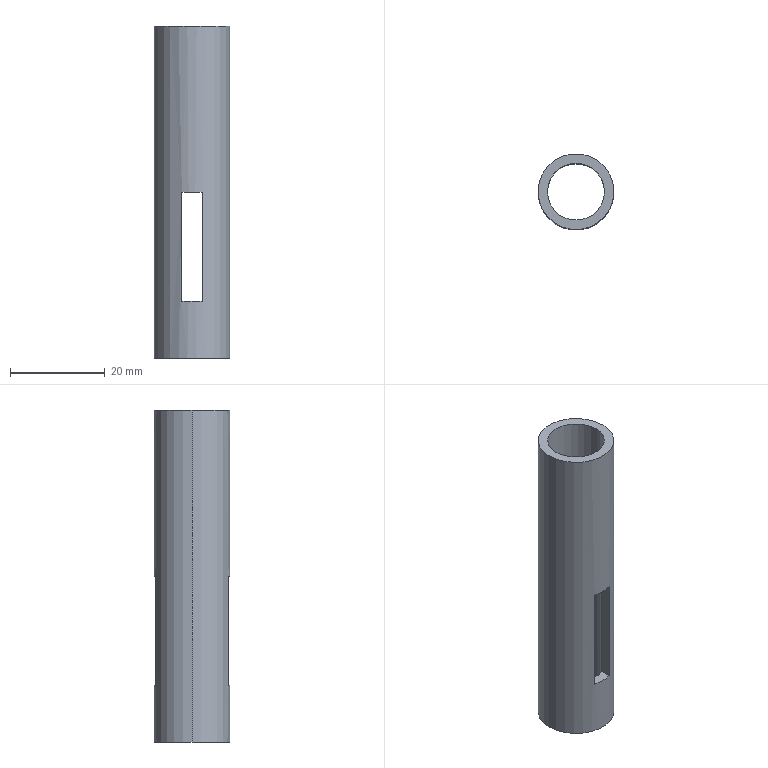Part | STEP file | Polisher lead screw | 1 solid | 14 faces | box 16 x 16 x 70 mm | volume 5755 mm3 | plane 10 | cylinder 4 | commonest cylinder face diameters 12 x2 16 x2
STEP:
#1=CARTESIAN_POINT('',(0.,0.,0.));
#2=DIRECTION('',(0.,0.,1.));
#3=DIRECTION('',(1.,0.,0.));
#4=AXIS2_PLACEMENT_3D('',#1,#2,#3);
#5=CARTESIAN_POINT('',(2.15,-5.602,-23.));
#6=VERTEX_POINT('',#5);
#7=CARTESIAN_POINT('',(-2.15,-5.602,-23.));
#8=VERTEX_POINT('',#7);
#9=CARTESIAN_POINT('',(0.,0.,-23.));
#10=DIRECTION('',(0.,0.,-1.));
#11=DIRECTION('',(-1.,0.,0.));
#12=AXIS2_PLACEMENT_3D('',#9,#10,#11);
#13=CIRCLE('',#12,6.);
#14=CARTESIAN_POINT('',(0.,0.,35.));
#15=DIRECTION('',(0.,0.,-1.));
#16=DIRECTION('',(-1.,0.,0.));
#17=AXIS2_PLACEMENT_3D('',#14,#15,#16);
#18=CYLINDRICAL_SURFACE('',#17,6.);
#19=CARTESIAN_POINT('',(0.,58.));
#20=DIRECTION('',(1.,0.));
#21=VECTOR('',#20,1.);
#22=LINE('',#19,#21);
#23=(GEOMETRIC_REPRESENTATION_CONTEXT(2)PARAMETRIC_REPRESENTATION_CONTEXT()REPRESENTATION_CONTEXT('',''));
#24=DEFINITIONAL_REPRESENTATION('',(#22),#23);
#25=PCURVE('',#18,#24);
#26=CARTESIAN_POINT('',(-2.15,-32.5,-23.));
#27=DIRECTION('',(0.,0.,-1.));
#28=DIRECTION('',(-1.,0.,0.));
#29=AXIS2_PLACEMENT_3D('',#26,#27,#28);
#30=PLANE('',#29);
#31=CARTESIAN_POINT('',(-2.15,32.5));
#32=DIRECTION('',(1.,0.));
#33=AXIS2_PLACEMENT_2D('',#31,#32);
#34=CIRCLE('',#33,6.);
#35=(GEOMETRIC_REPRESENTATION_CONTEXT(2)PARAMETRIC_REPRESENTATION_CONTEXT()REPRESENTATION_CONTEXT('',''));
#36=DEFINITIONAL_REPRESENTATION('',(#34),#35);
#37=PCURVE('',#30,#36);
#38=SURFACE_CURVE('',#13,(#25,#37),.PCURVE_S1.);
#39=EDGE_CURVE('',#6,#8,#38,.T.);
#40=ORIENTED_EDGE('',*,*,#39,.T.);
#41=CARTESIAN_POINT('',(-2.15,-5.602,0.));
#42=VERTEX_POINT('',#41);
#43=CARTESIAN_POINT('',(-2.15,-5.602,35.));
#44=DIRECTION('',(0.,0.,1.));
#45=VECTOR('',#44,1.);
#46=LINE('',#43,#45);
#47=CARTESIAN_POINT('',(5.079,0.));
#48=DIRECTION('',(0.,-1.));
#49=VECTOR('',#48,1.);
#50=LINE('',#47,#49);
#51=(GEOMETRIC_REPRESENTATION_CONTEXT(2)PARAMETRIC_REPRESENTATION_CONTEXT()REPRESENTATION_CONTEXT('',''));
#52=DEFINITIONAL_REPRESENTATION('',(#50),#51);
#53=PCURVE('',#18,#52);
#54=CARTESIAN_POINT('',(-2.15,-32.5,0.));
#55=DIRECTION('',(-1.,0.,0.));
#56=DIRECTION('',(0.,0.,1.));
#57=AXIS2_PLACEMENT_3D('',#54,#55,#56);
#58=PLANE('',#57);
#59=CARTESIAN_POINT('',(35.,26.898));
#60=DIRECTION('',(1.,0.));
#61=VECTOR('',#60,1.);
#62=LINE('',#59,#61);
#63=(GEOMETRIC_REPRESENTATION_CONTEXT(2)PARAMETRIC_REPRESENTATION_CONTEXT()REPRESENTATION_CONTEXT('',''));
#64=DEFINITIONAL_REPRESENTATION('',(#62),#63);
#65=PCURVE('',#58,#64);
#66=SURFACE_CURVE('',#46,(#53,#65),.PCURVE_S1.);
#67=EDGE_CURVE('',#8,#42,#66,.T.);
#68=ORIENTED_EDGE('',*,*,#67,.T.);
#69=CARTESIAN_POINT('',(2.15,-5.602,0.));
#70=VERTEX_POINT('',#69);
#71=CARTESIAN_POINT('',(0.,0.,0.));
#72=DIRECTION('',(0.,0.,1.));
#73=DIRECTION('',(1.,0.,0.));
#74=AXIS2_PLACEMENT_3D('',#71,#72,#73);
#75=CIRCLE('',#74,6.);
#76=CARTESIAN_POINT('',(9.425,35.));
#77=DIRECTION('',(-1.,0.));
#78=VECTOR('',#77,1.);
#79=LINE('',#76,#78);
#80=(GEOMETRIC_REPRESENTATION_CONTEXT(2)PARAMETRIC_REPRESENTATION_CONTEXT()REPRESENTATION_CONTEXT('',''));
#81=DEFINITIONAL_REPRESENTATION('',(#79),#80);
#82=PCURVE('',#18,#81);
#83=CARTESIAN_POINT('',(-2.15,-32.5,0.));
#84=DIRECTION('',(0.,0.,1.));
#85=DIRECTION('',(1.,0.,0.));
#86=AXIS2_PLACEMENT_3D('',#83,#84,#85);
#87=PLANE('',#86);
#88=CARTESIAN_POINT('',(2.15,32.5));
#89=DIRECTION('',(1.,0.));
#90=AXIS2_PLACEMENT_2D('',#88,#89);
#91=CIRCLE('',#90,6.);
#92=(GEOMETRIC_REPRESENTATION_CONTEXT(2)PARAMETRIC_REPRESENTATION_CONTEXT()REPRESENTATION_CONTEXT('',''));
#93=DEFINITIONAL_REPRESENTATION('',(#91),#92);
#94=PCURVE('',#87,#93);
#95=SURFACE_CURVE('',#75,(#82,#94),.PCURVE_S1.);
#96=EDGE_CURVE('',#42,#70,#95,.T.);
#97=ORIENTED_EDGE('',*,*,#96,.T.);
#98=CARTESIAN_POINT('',(2.15,-5.602,35.));
#99=DIRECTION('',(0.,0.,-1.));
#100=VECTOR('',#99,1.);
#101=LINE('',#98,#100);
#102=CARTESIAN_POINT('',(4.346,0.));
#103=DIRECTION('',(0.,1.));
#104=VECTOR('',#103,1.);
#105=LINE('',#102,#104);
#106=(GEOMETRIC_REPRESENTATION_CONTEXT(2)PARAMETRIC_REPRESENTATION_CONTEXT()REPRESENTATION_CONTEXT('',''));
#107=DEFINITIONAL_REPRESENTATION('',(#105),#106);
#108=PCURVE('',#18,#107);
#109=CARTESIAN_POINT('',(2.15,-32.5,0.));
#110=DIRECTION('',(1.,0.,0.));
#111=DIRECTION('',(0.,0.,-1.));
#112=AXIS2_PLACEMENT_3D('',#109,#110,#111);
#113=PLANE('',#112);
#114=CARTESIAN_POINT('',(-35.,26.898));
#115=DIRECTION('',(1.,0.));
#116=VECTOR('',#115,1.);
#117=LINE('',#114,#116);
#118=(GEOMETRIC_REPRESENTATION_CONTEXT(2)PARAMETRIC_REPRESENTATION_CONTEXT()REPRESENTATION_CONTEXT('',''));
#119=DEFINITIONAL_REPRESENTATION('',(#117),#118);
#120=PCURVE('',#113,#119);
#121=SURFACE_CURVE('',#101,(#108,#120),.PCURVE_S1.);
#122=EDGE_CURVE('',#70,#6,#121,.T.);
#123=ORIENTED_EDGE('',*,*,#122,.T.);
#124=EDGE_LOOP('',(#40,#68,#97,#123));
#125=FACE_BOUND('',#124,.F.);
#126=CARTESIAN_POINT('',(-6.,0.,35.));
#127=VERTEX_POINT('',#126);
#128=CARTESIAN_POINT('',(-6.,0.,-35.));
#129=VERTEX_POINT('',#128);
#130=CARTESIAN_POINT('',(-6.,0.,35.));
#131=DIRECTION('',(0.,0.,-1.));
#132=VECTOR('',#131,1.);
#133=LINE('',#130,#132);
#134=CARTESIAN_POINT('',(6.283,0.));
#135=DIRECTION('',(0.,1.));
#136=VECTOR('',#135,1.);
#137=LINE('',#134,#136);
#138=(GEOMETRIC_REPRESENTATION_CONTEXT(2)PARAMETRIC_REPRESENTATION_CONTEXT()REPRESENTATION_CONTEXT('',''));
#139=DEFINITIONAL_REPRESENTATION('',(#137),#138);
#140=PCURVE('',#18,#139);
#141=CARTESIAN_POINT('',(0.,0.,35.));
#142=DIRECTION('',(0.,0.,-1.));
#143=DIRECTION('',(-1.,0.,0.));
#144=AXIS2_PLACEMENT_3D('',#141,#142,#143);
#145=CYLINDRICAL_SURFACE('',#144,6.);
#146=CARTESIAN_POINT('',(0.,0.));
#147=DIRECTION('',(0.,1.));
#148=VECTOR('',#147,1.);
#149=LINE('',#146,#148);
#150=(GEOMETRIC_REPRESENTATION_CONTEXT(2)PARAMETRIC_REPRESENTATION_CONTEXT()REPRESENTATION_CONTEXT('',''));
#151=DEFINITIONAL_REPRESENTATION('',(#149),#150);
#152=PCURVE('',#145,#151);
#153=SURFACE_CURVE('',#133,(#140,#152),.PCURVE_S1.);
#154=EDGE_CURVE('',#127,#129,#153,.T.);
#155=ORIENTED_EDGE('',*,*,#154,.T.);
#156=CARTESIAN_POINT('',(6.,0.,-35.));
#157=VERTEX_POINT('',#156);
#158=CARTESIAN_POINT('',(0.,0.,-35.));
#159=DIRECTION('',(0.,0.,1.));
#160=DIRECTION('',(1.,0.,0.));
#161=AXIS2_PLACEMENT_3D('',#158,#159,#160);
#162=CIRCLE('',#161,6.);
#163=CARTESIAN_POINT('',(9.425,70.));
#164=DIRECTION('',(-1.,0.));
#165=VECTOR('',#164,1.);
#166=LINE('',#163,#165);
#167=(GEOMETRIC_REPRESENTATION_CONTEXT(2)PARAMETRIC_REPRESENTATION_CONTEXT()REPRESENTATION_CONTEXT('',''));
#168=DEFINITIONAL_REPRESENTATION('',(#166),#167);
#169=PCURVE('',#18,#168);
#170=CARTESIAN_POINT('',(0.,0.,-35.));
#171=DIRECTION('',(0.,0.,1.));
#172=DIRECTION('',(1.,0.,0.));
#173=AXIS2_PLACEMENT_3D('',#170,#171,#172);
#174=PLANE('',#173);
#175=CARTESIAN_POINT('',(0.,0.));
#176=DIRECTION('',(1.,0.));
#177=AXIS2_PLACEMENT_2D('',#175,#176);
#178=CIRCLE('',#177,6.);
#179=(GEOMETRIC_REPRESENTATION_CONTEXT(2)PARAMETRIC_REPRESENTATION_CONTEXT()REPRESENTATION_CONTEXT('',''));
#180=DEFINITIONAL_REPRESENTATION('',(#178),#179);
#181=PCURVE('',#174,#180);
#182=SURFACE_CURVE('',#162,(#169,#181),.PCURVE_S1.);
#183=EDGE_CURVE('',#129,#157,#182,.T.);
#184=ORIENTED_EDGE('',*,*,#183,.T.);
#185=CARTESIAN_POINT('',(6.,0.,35.));
#186=VERTEX_POINT('',#185);
#187=CARTESIAN_POINT('',(6.,0.,35.));
#188=DIRECTION('',(0.,0.,-1.));
#189=VECTOR('',#188,1.);
#190=LINE('',#187,#189);
#191=CARTESIAN_POINT('',(3.142,0.));
#192=DIRECTION('',(0.,1.));
#193=VECTOR('',#192,1.);
#194=LINE('',#191,#193);
#195=(GEOMETRIC_REPRESENTATION_CONTEXT(2)PARAMETRIC_REPRESENTATION_CONTEXT()REPRESENTATION_CONTEXT('',''));
#196=DEFINITIONAL_REPRESENTATION('',(#194),#195);
#197=PCURVE('',#18,#196);
#198=CARTESIAN_POINT('',(3.142,0.));
#199=DIRECTION('',(0.,1.));
#200=VECTOR('',#199,1.);
#201=LINE('',#198,#200);
#202=(GEOMETRIC_REPRESENTATION_CONTEXT(2)PARAMETRIC_REPRESENTATION_CONTEXT()REPRESENTATION_CONTEXT('',''));
#203=DEFINITIONAL_REPRESENTATION('',(#201),#202);
#204=PCURVE('',#145,#203);
#205=SURFACE_CURVE('',#190,(#197,#204),.PCURVE_S1.);
#206=EDGE_CURVE('',#186,#157,#205,.T.);
#207=ORIENTED_EDGE('',*,*,#206,.F.);
#208=CARTESIAN_POINT('',(0.,0.,35.));
#209=DIRECTION('',(0.,0.,1.));
#210=DIRECTION('',(1.,0.,0.));
#211=AXIS2_PLACEMENT_3D('',#208,#209,#210);
#212=CIRCLE('',#211,6.);
#213=CARTESIAN_POINT('',(9.425,0.));
#214=DIRECTION('',(-1.,0.));
#215=VECTOR('',#214,1.);
#216=LINE('',#213,#215);
#217=(GEOMETRIC_REPRESENTATION_CONTEXT(2)PARAMETRIC_REPRESENTATION_CONTEXT()REPRESENTATION_CONTEXT('',''));
#218=DEFINITIONAL_REPRESENTATION('',(#216),#217);
#219=PCURVE('',#18,#218);
#220=CARTESIAN_POINT('',(0.,0.,35.));
#221=DIRECTION('',(0.,0.,1.));
#222=DIRECTION('',(1.,0.,0.));
#223=AXIS2_PLACEMENT_3D('',#220,#221,#222);
#224=PLANE('',#223);
#225=CARTESIAN_POINT('',(0.,0.));
#226=DIRECTION('',(1.,0.));
#227=AXIS2_PLACEMENT_2D('',#225,#226);
#228=CIRCLE('',#227,6.);
#229=(GEOMETRIC_REPRESENTATION_CONTEXT(2)PARAMETRIC_REPRESENTATION_CONTEXT()REPRESENTATION_CONTEXT('',''));
#230=DEFINITIONAL_REPRESENTATION('',(#228),#229);
#231=PCURVE('',#224,#230);
#232=SURFACE_CURVE('',#212,(#219,#231),.PCURVE_S1.);
#233=EDGE_CURVE('',#127,#186,#232,.T.);
#234=ORIENTED_EDGE('',*,*,#233,.F.);
#235=EDGE_LOOP('',(#155,#184,#207,#234));
#236=FACE_BOUND('',#235,.F.);
#237=ADVANCED_FACE('',(#125,#236),#18,.F.);
#238=CARTESIAN_POINT('',(-2.15,7.706,-23.));
#239=VERTEX_POINT('',#238);
#240=CARTESIAN_POINT('',(2.15,7.706,-23.));
#241=VERTEX_POINT('',#240);
#242=CARTESIAN_POINT('',(0.,0.,-23.));
#243=DIRECTION('',(0.,0.,-1.));
#244=DIRECTION('',(-1.,0.,0.));
#245=AXIS2_PLACEMENT_3D('',#242,#243,#244);
#246=CIRCLE('',#245,8.);
#247=CARTESIAN_POINT('',(0.,0.,35.));
#248=DIRECTION('',(0.,0.,-1.));
#249=DIRECTION('',(-1.,0.,0.));
#250=AXIS2_PLACEMENT_3D('',#247,#248,#249);
#251=CYLINDRICAL_SURFACE('',#250,8.);
#252=CARTESIAN_POINT('',(0.,58.));
#253=DIRECTION('',(1.,0.));
#254=VECTOR('',#253,1.);
#255=LINE('',#252,#254);
#256=(GEOMETRIC_REPRESENTATION_CONTEXT(2)PARAMETRIC_REPRESENTATION_CONTEXT()REPRESENTATION_CONTEXT('',''));
#257=DEFINITIONAL_REPRESENTATION('',(#255),#256);
#258=PCURVE('',#251,#257);
#259=CARTESIAN_POINT('',(-2.15,-32.5,-23.));
#260=DIRECTION('',(0.,0.,-1.));
#261=DIRECTION('',(-1.,0.,0.));
#262=AXIS2_PLACEMENT_3D('',#259,#260,#261);
#263=PLANE('',#262);
#264=CARTESIAN_POINT('',(-2.15,32.5));
#265=DIRECTION('',(1.,0.));
#266=AXIS2_PLACEMENT_2D('',#264,#265);
#267=CIRCLE('',#266,8.);
#268=(GEOMETRIC_REPRESENTATION_CONTEXT(2)PARAMETRIC_REPRESENTATION_CONTEXT()REPRESENTATION_CONTEXT('',''));
#269=DEFINITIONAL_REPRESENTATION('',(#267),#268);
#270=PCURVE('',#263,#269);
#271=SURFACE_CURVE('',#246,(#258,#270),.PCURVE_S1.);
#272=EDGE_CURVE('',#239,#241,#271,.T.);
#273=ORIENTED_EDGE('',*,*,#272,.T.);
#274=CARTESIAN_POINT('',(2.15,7.706,0.));
#275=VERTEX_POINT('',#274);
#276=CARTESIAN_POINT('',(2.15,7.706,35.));
#277=DIRECTION('',(0.,0.,1.));
#278=VECTOR('',#277,1.);
#279=LINE('',#276,#278);
#280=CARTESIAN_POINT('',(1.843,0.));
#281=DIRECTION('',(0.,-1.));
#282=VECTOR('',#281,1.);
#283=LINE('',#280,#282);
#284=(GEOMETRIC_REPRESENTATION_CONTEXT(2)PARAMETRIC_REPRESENTATION_CONTEXT()REPRESENTATION_CONTEXT('',''));
#285=DEFINITIONAL_REPRESENTATION('',(#283),#284);
#286=PCURVE('',#251,#285);
#287=CARTESIAN_POINT('',(2.15,-32.5,0.));
#288=DIRECTION('',(1.,0.,0.));
#289=DIRECTION('',(0.,0.,-1.));
#290=AXIS2_PLACEMENT_3D('',#287,#288,#289);
#291=PLANE('',#290);
#292=CARTESIAN_POINT('',(-35.,40.206));
#293=DIRECTION('',(-1.,0.));
#294=VECTOR('',#293,1.);
#295=LINE('',#292,#294);
#296=(GEOMETRIC_REPRESENTATION_CONTEXT(2)PARAMETRIC_REPRESENTATION_CONTEXT()REPRESENTATION_CONTEXT('',''));
#297=DEFINITIONAL_REPRESENTATION('',(#295),#296);
#298=PCURVE('',#291,#297);
#299=SURFACE_CURVE('',#279,(#286,#298),.PCURVE_S1.);
#300=EDGE_CURVE('',#241,#275,#299,.T.);
#301=ORIENTED_EDGE('',*,*,#300,.T.);
#302=CARTESIAN_POINT('',(-2.15,7.706,0.));
#303=VERTEX_POINT('',#302);
#304=CARTESIAN_POINT('',(0.,0.,0.));
#305=DIRECTION('',(0.,0.,1.));
#306=DIRECTION('',(1.,0.,0.));
#307=AXIS2_PLACEMENT_3D('',#304,#305,#306);
#308=CIRCLE('',#307,8.);
#309=CARTESIAN_POINT('',(3.142,35.));
#310=DIRECTION('',(-1.,0.));
#311=VECTOR('',#310,1.);
#312=LINE('',#309,#311);
#313=(GEOMETRIC_REPRESENTATION_CONTEXT(2)PARAMETRIC_REPRESENTATION_CONTEXT()REPRESENTATION_CONTEXT('',''));
#314=DEFINITIONAL_REPRESENTATION('',(#312),#313);
#315=PCURVE('',#251,#314);
#316=CARTESIAN_POINT('',(-2.15,-32.5,0.));
#317=DIRECTION('',(0.,0.,1.));
#318=DIRECTION('',(1.,0.,0.));
#319=AXIS2_PLACEMENT_3D('',#316,#317,#318);
#320=PLANE('',#319);
#321=CARTESIAN_POINT('',(2.15,32.5));
#322=DIRECTION('',(1.,0.));
#323=AXIS2_PLACEMENT_2D('',#321,#322);
#324=CIRCLE('',#323,8.);
#325=(GEOMETRIC_REPRESENTATION_CONTEXT(2)PARAMETRIC_REPRESENTATION_CONTEXT()REPRESENTATION_CONTEXT('',''));
#326=DEFINITIONAL_REPRESENTATION('',(#324),#325);
#327=PCURVE('',#320,#326);
#328=SURFACE_CURVE('',#308,(#315,#327),.PCURVE_S1.);
#329=EDGE_CURVE('',#275,#303,#328,.T.);
#330=ORIENTED_EDGE('',*,*,#329,.T.);
#331=CARTESIAN_POINT('',(-2.15,7.706,35.));
#332=DIRECTION('',(0.,0.,-1.));
#333=VECTOR('',#332,1.);
#334=LINE('',#331,#333);
#335=CARTESIAN_POINT('',(1.299,0.));
#336=DIRECTION('',(0.,1.));
#337=VECTOR('',#336,1.);
#338=LINE('',#335,#337);
#339=(GEOMETRIC_REPRESENTATION_CONTEXT(2)PARAMETRIC_REPRESENTATION_CONTEXT()REPRESENTATION_CONTEXT('',''));
#340=DEFINITIONAL_REPRESENTATION('',(#338),#339);
#341=PCURVE('',#251,#340);
#342=CARTESIAN_POINT('',(-2.15,-32.5,0.));
#343=DIRECTION('',(-1.,0.,0.));
#344=DIRECTION('',(0.,0.,1.));
#345=AXIS2_PLACEMENT_3D('',#342,#343,#344);
#346=PLANE('',#345);
#347=CARTESIAN_POINT('',(35.,40.206));
#348=DIRECTION('',(-1.,0.));
#349=VECTOR('',#348,1.);
#350=LINE('',#347,#349);
#351=(GEOMETRIC_REPRESENTATION_CONTEXT(2)PARAMETRIC_REPRESENTATION_CONTEXT()REPRESENTATION_CONTEXT('',''));
#352=DEFINITIONAL_REPRESENTATION('',(#350),#351);
#353=PCURVE('',#346,#352);
#354=SURFACE_CURVE('',#334,(#341,#353),.PCURVE_S1.);
#355=EDGE_CURVE('',#303,#239,#354,.T.);
#356=ORIENTED_EDGE('',*,*,#355,.T.);
#357=EDGE_LOOP('',(#273,#301,#330,#356));
#358=FACE_BOUND('',#357,.T.);
#359=CARTESIAN_POINT('',(8.,0.,35.));
#360=VERTEX_POINT('',#359);
#361=CARTESIAN_POINT('',(-8.,0.,35.));
#362=VERTEX_POINT('',#361);
#363=CARTESIAN_POINT('',(0.,0.,35.));
#364=DIRECTION('',(0.,0.,1.));
#365=DIRECTION('',(1.,0.,0.));
#366=AXIS2_PLACEMENT_3D('',#363,#364,#365);
#367=CIRCLE('',#366,8.);
#368=CARTESIAN_POINT('',(3.142,0.));
#369=DIRECTION('',(-1.,0.));
#370=VECTOR('',#369,1.);
#371=LINE('',#368,#370);
#372=(GEOMETRIC_REPRESENTATION_CONTEXT(2)PARAMETRIC_REPRESENTATION_CONTEXT()REPRESENTATION_CONTEXT('',''));
#373=DEFINITIONAL_REPRESENTATION('',(#371),#372);
#374=PCURVE('',#251,#373);
#375=CARTESIAN_POINT('',(0.,0.));
#376=DIRECTION('',(1.,0.));
#377=AXIS2_PLACEMENT_2D('',#375,#376);
#378=CIRCLE('',#377,8.);
#379=(GEOMETRIC_REPRESENTATION_CONTEXT(2)PARAMETRIC_REPRESENTATION_CONTEXT()REPRESENTATION_CONTEXT('',''));
#380=DEFINITIONAL_REPRESENTATION('',(#378),#379);
#381=PCURVE('',#224,#380);
#382=SURFACE_CURVE('',#367,(#374,#381),.PCURVE_S1.);
#383=EDGE_CURVE('',#360,#362,#382,.T.);
#384=ORIENTED_EDGE('',*,*,#383,.F.);
#385=CARTESIAN_POINT('',(8.,0.,-35.));
#386=VERTEX_POINT('',#385);
#387=CARTESIAN_POINT('',(8.,0.,35.));
#388=DIRECTION('',(0.,0.,-1.));
#389=VECTOR('',#388,1.);
#390=LINE('',#387,#389);
#391=CARTESIAN_POINT('',(3.142,0.));
#392=DIRECTION('',(0.,1.));
#393=VECTOR('',#392,1.);
#394=LINE('',#391,#393);
#395=(GEOMETRIC_REPRESENTATION_CONTEXT(2)PARAMETRIC_REPRESENTATION_CONTEXT()REPRESENTATION_CONTEXT('',''));
#396=DEFINITIONAL_REPRESENTATION('',(#394),#395);
#397=PCURVE('',#251,#396);
#398=CARTESIAN_POINT('',(0.,0.,35.));
#399=DIRECTION('',(0.,0.,-1.));
#400=DIRECTION('',(-1.,0.,0.));
#401=AXIS2_PLACEMENT_3D('',#398,#399,#400);
#402=CYLINDRICAL_SURFACE('',#401,8.);
#403=CARTESIAN_POINT('',(3.142,0.));
#404=DIRECTION('',(0.,1.));
#405=VECTOR('',#404,1.);
#406=LINE('',#403,#405);
#407=(GEOMETRIC_REPRESENTATION_CONTEXT(2)PARAMETRIC_REPRESENTATION_CONTEXT()REPRESENTATION_CONTEXT('',''));
#408=DEFINITIONAL_REPRESENTATION('',(#406),#407);
#409=PCURVE('',#402,#408);
#410=SURFACE_CURVE('',#390,(#397,#409),.PCURVE_S1.);
#411=EDGE_CURVE('',#360,#386,#410,.T.);
#412=ORIENTED_EDGE('',*,*,#411,.T.);
#413=CARTESIAN_POINT('',(-8.,0.,-35.));
#414=VERTEX_POINT('',#413);
#415=CARTESIAN_POINT('',(0.,0.,-35.));
#416=DIRECTION('',(0.,0.,1.));
#417=DIRECTION('',(1.,0.,0.));
#418=AXIS2_PLACEMENT_3D('',#415,#416,#417);
#419=CIRCLE('',#418,8.);
#420=CARTESIAN_POINT('',(3.142,70.));
#421=DIRECTION('',(-1.,0.));
#422=VECTOR('',#421,1.);
#423=LINE('',#420,#422);
#424=(GEOMETRIC_REPRESENTATION_CONTEXT(2)PARAMETRIC_REPRESENTATION_CONTEXT()REPRESENTATION_CONTEXT('',''));
#425=DEFINITIONAL_REPRESENTATION('',(#423),#424);
#426=PCURVE('',#251,#425);
#427=CARTESIAN_POINT('',(0.,0.));
#428=DIRECTION('',(1.,0.));
#429=AXIS2_PLACEMENT_2D('',#427,#428);
#430=CIRCLE('',#429,8.);
#431=(GEOMETRIC_REPRESENTATION_CONTEXT(2)PARAMETRIC_REPRESENTATION_CONTEXT()REPRESENTATION_CONTEXT('',''));
#432=DEFINITIONAL_REPRESENTATION('',(#430),#431);
#433=PCURVE('',#174,#432);
#434=SURFACE_CURVE('',#419,(#426,#433),.PCURVE_S1.);
#435=EDGE_CURVE('',#386,#414,#434,.T.);
#436=ORIENTED_EDGE('',*,*,#435,.T.);
#437=CARTESIAN_POINT('',(-8.,0.,35.));
#438=DIRECTION('',(0.,0.,-1.));
#439=VECTOR('',#438,1.);
#440=LINE('',#437,#439);
#441=CARTESIAN_POINT('',(0.,0.));
#442=DIRECTION('',(0.,1.));
#443=VECTOR('',#442,1.);
#444=LINE('',#441,#443);
#445=(GEOMETRIC_REPRESENTATION_CONTEXT(2)PARAMETRIC_REPRESENTATION_CONTEXT()REPRESENTATION_CONTEXT('',''));
#446=DEFINITIONAL_REPRESENTATION('',(#444),#445);
#447=PCURVE('',#251,#446);
#448=CARTESIAN_POINT('',(6.283,0.));
#449=DIRECTION('',(0.,1.));
#450=VECTOR('',#449,1.);
#451=LINE('',#448,#450);
#452=(GEOMETRIC_REPRESENTATION_CONTEXT(2)PARAMETRIC_REPRESENTATION_CONTEXT()REPRESENTATION_CONTEXT('',''));
#453=DEFINITIONAL_REPRESENTATION('',(#451),#452);
#454=PCURVE('',#402,#453);
#455=SURFACE_CURVE('',#440,(#447,#454),.PCURVE_S1.);
#456=EDGE_CURVE('',#362,#414,#455,.T.);
#457=ORIENTED_EDGE('',*,*,#456,.F.);
#458=EDGE_LOOP('',(#384,#412,#436,#457));
#459=FACE_BOUND('',#458,.T.);
#460=ADVANCED_FACE('',(#358,#459),#251,.T.);
#461=CARTESIAN_POINT('',(0.,0.,35.));
#462=DIRECTION('',(0.,0.,1.));
#463=DIRECTION('',(1.,0.,0.));
#464=AXIS2_PLACEMENT_3D('',#461,#462,#463);
#465=CIRCLE('',#464,8.);
#466=CARTESIAN_POINT('',(0.,0.));
#467=DIRECTION('',(1.,0.));
#468=AXIS2_PLACEMENT_2D('',#466,#467);
#469=CIRCLE('',#468,8.);
#470=(GEOMETRIC_REPRESENTATION_CONTEXT(2)PARAMETRIC_REPRESENTATION_CONTEXT()REPRESENTATION_CONTEXT('',''));
#471=DEFINITIONAL_REPRESENTATION('',(#469),#470);
#472=PCURVE('',#224,#471);
#473=CARTESIAN_POINT('',(9.425,0.));
#474=DIRECTION('',(-1.,0.));
#475=VECTOR('',#474,1.);
#476=LINE('',#473,#475);
#477=(GEOMETRIC_REPRESENTATION_CONTEXT(2)PARAMETRIC_REPRESENTATION_CONTEXT()REPRESENTATION_CONTEXT('',''));
#478=DEFINITIONAL_REPRESENTATION('',(#476),#477);
#479=PCURVE('',#402,#478);
#480=SURFACE_CURVE('',#465,(#472,#479),.PCURVE_S1.);
#481=EDGE_CURVE('',#362,#360,#480,.T.);
#482=ORIENTED_EDGE('',*,*,#481,.T.);
#483=ORIENTED_EDGE('',*,*,#383,.T.);
#484=EDGE_LOOP('',(#482,#483));
#485=FACE_BOUND('',#484,.T.);
#486=ORIENTED_EDGE('',*,*,#233,.F.);
#487=CARTESIAN_POINT('',(0.,0.,35.));
#488=DIRECTION('',(0.,0.,1.));
#489=DIRECTION('',(1.,0.,0.));
#490=AXIS2_PLACEMENT_3D('',#487,#488,#489);
#491=CIRCLE('',#490,6.);
#492=CARTESIAN_POINT('',(0.,0.));
#493=DIRECTION('',(1.,0.));
#494=AXIS2_PLACEMENT_2D('',#492,#493);
#495=CIRCLE('',#494,6.);
#496=(GEOMETRIC_REPRESENTATION_CONTEXT(2)PARAMETRIC_REPRESENTATION_CONTEXT()REPRESENTATION_CONTEXT('',''));
#497=DEFINITIONAL_REPRESENTATION('',(#495),#496);
#498=PCURVE('',#224,#497);
#499=CARTESIAN_POINT('',(3.142,0.));
#500=DIRECTION('',(-1.,0.));
#501=VECTOR('',#500,1.);
#502=LINE('',#499,#501);
#503=(GEOMETRIC_REPRESENTATION_CONTEXT(2)PARAMETRIC_REPRESENTATION_CONTEXT()REPRESENTATION_CONTEXT('',''));
#504=DEFINITIONAL_REPRESENTATION('',(#502),#503);
#505=PCURVE('',#145,#504);
#506=SURFACE_CURVE('',#491,(#498,#505),.PCURVE_S1.);
#507=EDGE_CURVE('',#186,#127,#506,.T.);
#508=ORIENTED_EDGE('',*,*,#507,.F.);
#509=EDGE_LOOP('',(#486,#508));
#510=FACE_BOUND('',#509,.T.);
#511=ADVANCED_FACE('',(#485,#510),#224,.T.);
#512=CARTESIAN_POINT('',(0.,0.,-35.));
#513=DIRECTION('',(0.,0.,1.));
#514=DIRECTION('',(1.,0.,0.));
#515=AXIS2_PLACEMENT_3D('',#512,#513,#514);
#516=CIRCLE('',#515,8.);
#517=CARTESIAN_POINT('',(0.,0.));
#518=DIRECTION('',(1.,0.));
#519=AXIS2_PLACEMENT_2D('',#517,#518);
#520=CIRCLE('',#519,8.);
#521=(GEOMETRIC_REPRESENTATION_CONTEXT(2)PARAMETRIC_REPRESENTATION_CONTEXT()REPRESENTATION_CONTEXT('',''));
#522=DEFINITIONAL_REPRESENTATION('',(#520),#521);
#523=PCURVE('',#174,#522);
#524=CARTESIAN_POINT('',(9.425,70.));
#525=DIRECTION('',(-1.,0.));
#526=VECTOR('',#525,1.);
#527=LINE('',#524,#526);
#528=(GEOMETRIC_REPRESENTATION_CONTEXT(2)PARAMETRIC_REPRESENTATION_CONTEXT()REPRESENTATION_CONTEXT('',''));
#529=DEFINITIONAL_REPRESENTATION('',(#527),#528);
#530=PCURVE('',#402,#529);
#531=SURFACE_CURVE('',#516,(#523,#530),.PCURVE_S1.);
#532=EDGE_CURVE('',#414,#386,#531,.T.);
#533=ORIENTED_EDGE('',*,*,#532,.F.);
#534=ORIENTED_EDGE('',*,*,#435,.F.);
#535=EDGE_LOOP('',(#533,#534));
#536=FACE_BOUND('',#535,.T.);
#537=ORIENTED_EDGE('',*,*,#183,.T.);
#538=CARTESIAN_POINT('',(0.,0.,-35.));
#539=DIRECTION('',(0.,0.,1.));
#540=DIRECTION('',(1.,0.,0.));
#541=AXIS2_PLACEMENT_3D('',#538,#539,#540);
#542=CIRCLE('',#541,6.);
#543=CARTESIAN_POINT('',(0.,0.));
#544=DIRECTION('',(1.,0.));
#545=AXIS2_PLACEMENT_2D('',#543,#544);
#546=CIRCLE('',#545,6.);
#547=(GEOMETRIC_REPRESENTATION_CONTEXT(2)PARAMETRIC_REPRESENTATION_CONTEXT()REPRESENTATION_CONTEXT('',''));
#548=DEFINITIONAL_REPRESENTATION('',(#546),#547);
#549=PCURVE('',#174,#548);
#550=CARTESIAN_POINT('',(3.142,70.));
#551=DIRECTION('',(-1.,0.));
#552=VECTOR('',#551,1.);
#553=LINE('',#550,#552);
#554=(GEOMETRIC_REPRESENTATION_CONTEXT(2)PARAMETRIC_REPRESENTATION_CONTEXT()REPRESENTATION_CONTEXT('',''));
#555=DEFINITIONAL_REPRESENTATION('',(#553),#554);
#556=PCURVE('',#145,#555);
#557=SURFACE_CURVE('',#542,(#549,#556),.PCURVE_S1.);
#558=EDGE_CURVE('',#157,#129,#557,.T.);
#559=ORIENTED_EDGE('',*,*,#558,.T.);
#560=EDGE_LOOP('',(#537,#559));
#561=FACE_BOUND('',#560,.T.);
#562=ADVANCED_FACE('',(#536,#561),#174,.F.);
#563=ORIENTED_EDGE('',*,*,#411,.F.);
#564=ORIENTED_EDGE('',*,*,#481,.F.);
#565=ORIENTED_EDGE('',*,*,#456,.T.);
#566=ORIENTED_EDGE('',*,*,#532,.T.);
#567=EDGE_LOOP('',(#563,#564,#565,#566));
#568=FACE_BOUND('',#567,.T.);
#569=CARTESIAN_POINT('',(-2.15,-7.706,0.));
#570=VERTEX_POINT('',#569);
#571=CARTESIAN_POINT('',(2.15,-7.706,0.));
#572=VERTEX_POINT('',#571);
#573=CARTESIAN_POINT('',(0.,0.,0.));
#574=DIRECTION('',(0.,0.,1.));
#575=DIRECTION('',(1.,0.,0.));
#576=AXIS2_PLACEMENT_3D('',#573,#574,#575);
#577=CIRCLE('',#576,8.);
#578=CARTESIAN_POINT('',(9.425,35.));
#579=DIRECTION('',(-1.,0.));
#580=VECTOR('',#579,1.);
#581=LINE('',#578,#580);
#582=(GEOMETRIC_REPRESENTATION_CONTEXT(2)PARAMETRIC_REPRESENTATION_CONTEXT()REPRESENTATION_CONTEXT('',''));
#583=DEFINITIONAL_REPRESENTATION('',(#581),#582);
#584=PCURVE('',#402,#583);
#585=CARTESIAN_POINT('',(2.15,32.5));
#586=DIRECTION('',(1.,0.));
#587=AXIS2_PLACEMENT_2D('',#585,#586);
#588=CIRCLE('',#587,8.);
#589=(GEOMETRIC_REPRESENTATION_CONTEXT(2)PARAMETRIC_REPRESENTATION_CONTEXT()REPRESENTATION_CONTEXT('',''));
#590=DEFINITIONAL_REPRESENTATION('',(#588),#589);
#591=PCURVE('',#87,#590);
#592=SURFACE_CURVE('',#577,(#584,#591),.PCURVE_S1.);
#593=EDGE_CURVE('',#570,#572,#592,.T.);
#594=ORIENTED_EDGE('',*,*,#593,.T.);
#595=CARTESIAN_POINT('',(2.15,-7.706,-23.));
#596=VERTEX_POINT('',#595);
#597=CARTESIAN_POINT('',(2.15,-7.706,35.));
#598=DIRECTION('',(0.,0.,-1.));
#599=VECTOR('',#598,1.);
#600=LINE('',#597,#599);
#601=CARTESIAN_POINT('',(4.44,0.));
#602=DIRECTION('',(0.,1.));
#603=VECTOR('',#602,1.);
#604=LINE('',#601,#603);
#605=(GEOMETRIC_REPRESENTATION_CONTEXT(2)PARAMETRIC_REPRESENTATION_CONTEXT()REPRESENTATION_CONTEXT('',''));
#606=DEFINITIONAL_REPRESENTATION('',(#604),#605);
#607=PCURVE('',#402,#606);
#608=CARTESIAN_POINT('',(-35.,24.794));
#609=DIRECTION('',(1.,0.));
#610=VECTOR('',#609,1.);
#611=LINE('',#608,#610);
#612=(GEOMETRIC_REPRESENTATION_CONTEXT(2)PARAMETRIC_REPRESENTATION_CONTEXT()REPRESENTATION_CONTEXT('',''));
#613=DEFINITIONAL_REPRESENTATION('',(#611),#612);
#614=PCURVE('',#113,#613);
#615=SURFACE_CURVE('',#600,(#607,#614),.PCURVE_S1.);
#616=EDGE_CURVE('',#572,#596,#615,.T.);
#617=ORIENTED_EDGE('',*,*,#616,.T.);
#618=CARTESIAN_POINT('',(-2.15,-7.706,-23.));
#619=VERTEX_POINT('',#618);
#620=CARTESIAN_POINT('',(0.,0.,-23.));
#621=DIRECTION('',(0.,0.,-1.));
#622=DIRECTION('',(-1.,0.,0.));
#623=AXIS2_PLACEMENT_3D('',#620,#621,#622);
#624=CIRCLE('',#623,8.);
#625=CARTESIAN_POINT('',(0.,58.));
#626=DIRECTION('',(1.,0.));
#627=VECTOR('',#626,1.);
#628=LINE('',#625,#627);
#629=(GEOMETRIC_REPRESENTATION_CONTEXT(2)PARAMETRIC_REPRESENTATION_CONTEXT()REPRESENTATION_CONTEXT('',''));
#630=DEFINITIONAL_REPRESENTATION('',(#628),#629);
#631=PCURVE('',#402,#630);
#632=CARTESIAN_POINT('',(-2.15,32.5));
#633=DIRECTION('',(1.,0.));
#634=AXIS2_PLACEMENT_2D('',#632,#633);
#635=CIRCLE('',#634,8.);
#636=(GEOMETRIC_REPRESENTATION_CONTEXT(2)PARAMETRIC_REPRESENTATION_CONTEXT()REPRESENTATION_CONTEXT('',''));
#637=DEFINITIONAL_REPRESENTATION('',(#635),#636);
#638=PCURVE('',#30,#637);
#639=SURFACE_CURVE('',#624,(#631,#638),.PCURVE_S1.);
#640=EDGE_CURVE('',#596,#619,#639,.T.);
#641=ORIENTED_EDGE('',*,*,#640,.T.);
#642=CARTESIAN_POINT('',(-2.15,-7.706,35.));
#643=DIRECTION('',(0.,0.,1.));
#644=VECTOR('',#643,1.);
#645=LINE('',#642,#644);
#646=CARTESIAN_POINT('',(4.984,0.));
#647=DIRECTION('',(0.,-1.));
#648=VECTOR('',#647,1.);
#649=LINE('',#646,#648);
#650=(GEOMETRIC_REPRESENTATION_CONTEXT(2)PARAMETRIC_REPRESENTATION_CONTEXT()REPRESENTATION_CONTEXT('',''));
#651=DEFINITIONAL_REPRESENTATION('',(#649),#650);
#652=PCURVE('',#402,#651);
#653=CARTESIAN_POINT('',(35.,24.794));
#654=DIRECTION('',(1.,0.));
#655=VECTOR('',#654,1.);
#656=LINE('',#653,#655);
#657=(GEOMETRIC_REPRESENTATION_CONTEXT(2)PARAMETRIC_REPRESENTATION_CONTEXT()REPRESENTATION_CONTEXT('',''));
#658=DEFINITIONAL_REPRESENTATION('',(#656),#657);
#659=PCURVE('',#58,#658);
#660=SURFACE_CURVE('',#645,(#652,#659),.PCURVE_S1.);
#661=EDGE_CURVE('',#619,#570,#660,.T.);
#662=ORIENTED_EDGE('',*,*,#661,.T.);
#663=EDGE_LOOP('',(#594,#617,#641,#662));
#664=FACE_BOUND('',#663,.T.);
#665=ADVANCED_FACE('',(#568,#664),#402,.T.);
#666=ORIENTED_EDGE('',*,*,#558,.T.);
#667=ORIENTED_EDGE('',*,*,#154,.F.);
#668=ORIENTED_EDGE('',*,*,#507,.F.);
#669=ORIENTED_EDGE('',*,*,#206,.T.);
#670=EDGE_LOOP('',(#666,#667,#668,#669));
#671=FACE_BOUND('',#670,.F.);
#672=CARTESIAN_POINT('',(2.15,5.602,0.));
#673=VERTEX_POINT('',#672);
#674=CARTESIAN_POINT('',(-2.15,5.602,0.));
#675=VERTEX_POINT('',#674);
#676=CARTESIAN_POINT('',(0.,0.,0.));
#677=DIRECTION('',(0.,0.,1.));
#678=DIRECTION('',(1.,0.,0.));
#679=AXIS2_PLACEMENT_3D('',#676,#677,#678);
#680=CIRCLE('',#679,6.);
#681=CARTESIAN_POINT('',(3.142,35.));
#682=DIRECTION('',(-1.,0.));
#683=VECTOR('',#682,1.);
#684=LINE('',#681,#683);
#685=(GEOMETRIC_REPRESENTATION_CONTEXT(2)PARAMETRIC_REPRESENTATION_CONTEXT()REPRESENTATION_CONTEXT('',''));
#686=DEFINITIONAL_REPRESENTATION('',(#684),#685);
#687=PCURVE('',#145,#686);
#688=CARTESIAN_POINT('',(2.15,32.5));
#689=DIRECTION('',(1.,0.));
#690=AXIS2_PLACEMENT_2D('',#688,#689);
#691=CIRCLE('',#690,6.);
#692=(GEOMETRIC_REPRESENTATION_CONTEXT(2)PARAMETRIC_REPRESENTATION_CONTEXT()REPRESENTATION_CONTEXT('',''));
#693=DEFINITIONAL_REPRESENTATION('',(#691),#692);
#694=PCURVE('',#320,#693);
#695=SURFACE_CURVE('',#680,(#687,#694),.PCURVE_S1.);
#696=EDGE_CURVE('',#673,#675,#695,.T.);
#697=ORIENTED_EDGE('',*,*,#696,.T.);
#698=CARTESIAN_POINT('',(-2.15,5.602,-23.));
#699=VERTEX_POINT('',#698);
#700=CARTESIAN_POINT('',(-2.15,5.602,35.));
#701=DIRECTION('',(0.,0.,-1.));
#702=VECTOR('',#701,1.);
#703=LINE('',#700,#702);
#704=CARTESIAN_POINT('',(1.204,0.));
#705=DIRECTION('',(0.,1.));
#706=VECTOR('',#705,1.);
#707=LINE('',#704,#706);
#708=(GEOMETRIC_REPRESENTATION_CONTEXT(2)PARAMETRIC_REPRESENTATION_CONTEXT()REPRESENTATION_CONTEXT('',''));
#709=DEFINITIONAL_REPRESENTATION('',(#707),#708);
#710=PCURVE('',#145,#709);
#711=CARTESIAN_POINT('',(35.,38.102));
#712=DIRECTION('',(-1.,0.));
#713=VECTOR('',#712,1.);
#714=LINE('',#711,#713);
#715=(GEOMETRIC_REPRESENTATION_CONTEXT(2)PARAMETRIC_REPRESENTATION_CONTEXT()REPRESENTATION_CONTEXT('',''));
#716=DEFINITIONAL_REPRESENTATION('',(#714),#715);
#717=PCURVE('',#346,#716);
#718=SURFACE_CURVE('',#703,(#710,#717),.PCURVE_S1.);
#719=EDGE_CURVE('',#675,#699,#718,.T.);
#720=ORIENTED_EDGE('',*,*,#719,.T.);
#721=CARTESIAN_POINT('',(2.15,5.602,-23.));
#722=VERTEX_POINT('',#721);
#723=CARTESIAN_POINT('',(0.,0.,-23.));
#724=DIRECTION('',(0.,0.,-1.));
#725=DIRECTION('',(-1.,0.,0.));
#726=AXIS2_PLACEMENT_3D('',#723,#724,#725);
#727=CIRCLE('',#726,6.);
#728=CARTESIAN_POINT('',(0.,58.));
#729=DIRECTION('',(1.,0.));
#730=VECTOR('',#729,1.);
#731=LINE('',#728,#730);
#732=(GEOMETRIC_REPRESENTATION_CONTEXT(2)PARAMETRIC_REPRESENTATION_CONTEXT()REPRESENTATION_CONTEXT('',''));
#733=DEFINITIONAL_REPRESENTATION('',(#731),#732);
#734=PCURVE('',#145,#733);
#735=CARTESIAN_POINT('',(-2.15,32.5));
#736=DIRECTION('',(1.,0.));
#737=AXIS2_PLACEMENT_2D('',#735,#736);
#738=CIRCLE('',#737,6.);
#739=(GEOMETRIC_REPRESENTATION_CONTEXT(2)PARAMETRIC_REPRESENTATION_CONTEXT()REPRESENTATION_CONTEXT('',''));
#740=DEFINITIONAL_REPRESENTATION('',(#738),#739);
#741=PCURVE('',#263,#740);
#742=SURFACE_CURVE('',#727,(#734,#741),.PCURVE_S1.);
#743=EDGE_CURVE('',#699,#722,#742,.T.);
#744=ORIENTED_EDGE('',*,*,#743,.T.);
#745=CARTESIAN_POINT('',(2.15,5.602,35.));
#746=DIRECTION('',(0.,0.,1.));
#747=VECTOR('',#746,1.);
#748=LINE('',#745,#747);
#749=CARTESIAN_POINT('',(1.937,0.));
#750=DIRECTION('',(0.,-1.));
#751=VECTOR('',#750,1.);
#752=LINE('',#749,#751);
#753=(GEOMETRIC_REPRESENTATION_CONTEXT(2)PARAMETRIC_REPRESENTATION_CONTEXT()REPRESENTATION_CONTEXT('',''));
#754=DEFINITIONAL_REPRESENTATION('',(#752),#753);
#755=PCURVE('',#145,#754);
#756=CARTESIAN_POINT('',(-35.,38.102));
#757=DIRECTION('',(-1.,0.));
#758=VECTOR('',#757,1.);
#759=LINE('',#756,#758);
#760=(GEOMETRIC_REPRESENTATION_CONTEXT(2)PARAMETRIC_REPRESENTATION_CONTEXT()REPRESENTATION_CONTEXT('',''));
#761=DEFINITIONAL_REPRESENTATION('',(#759),#760);
#762=PCURVE('',#291,#761);
#763=SURFACE_CURVE('',#748,(#755,#762),.PCURVE_S1.);
#764=EDGE_CURVE('',#722,#673,#763,.T.);
#765=ORIENTED_EDGE('',*,*,#764,.T.);
#766=EDGE_LOOP('',(#697,#720,#744,#765));
#767=FACE_BOUND('',#766,.F.);
#768=ADVANCED_FACE('',(#671,#767),#145,.F.);
#769=CARTESIAN_POINT('',(2.15,-32.5,-23.));
#770=DIRECTION('',(0.,1.,0.));
#771=VECTOR('',#770,1.);
#772=LINE('',#769,#771);
#773=CARTESIAN_POINT('',(-4.3,0.));
#774=DIRECTION('',(0.,1.));
#775=VECTOR('',#774,1.);
#776=LINE('',#773,#775);
#777=(GEOMETRIC_REPRESENTATION_CONTEXT(2)PARAMETRIC_REPRESENTATION_CONTEXT()REPRESENTATION_CONTEXT('',''));
#778=DEFINITIONAL_REPRESENTATION('',(#776),#777);
#779=PCURVE('',#30,#778);
#780=CARTESIAN_POINT('',(23.,0.));
#781=DIRECTION('',(0.,1.));
#782=VECTOR('',#781,1.);
#783=LINE('',#780,#782);
#784=(GEOMETRIC_REPRESENTATION_CONTEXT(2)PARAMETRIC_REPRESENTATION_CONTEXT()REPRESENTATION_CONTEXT('',''));
#785=DEFINITIONAL_REPRESENTATION('',(#783),#784);
#786=PCURVE('',#113,#785);
#787=SURFACE_CURVE('',#772,(#779,#786),.PCURVE_S1.);
#788=EDGE_CURVE('',#596,#6,#787,.T.);
#789=ORIENTED_EDGE('',*,*,#788,.T.);
#790=ORIENTED_EDGE('',*,*,#39,.T.);
#791=CARTESIAN_POINT('',(-2.15,-32.5,-23.));
#792=DIRECTION('',(0.,1.,0.));
#793=VECTOR('',#792,1.);
#794=LINE('',#791,#793);
#795=CARTESIAN_POINT('',(0.,0.));
#796=DIRECTION('',(0.,1.));
#797=VECTOR('',#796,1.);
#798=LINE('',#795,#797);
#799=(GEOMETRIC_REPRESENTATION_CONTEXT(2)PARAMETRIC_REPRESENTATION_CONTEXT()REPRESENTATION_CONTEXT('',''));
#800=DEFINITIONAL_REPRESENTATION('',(#798),#799);
#801=PCURVE('',#30,#800);
#802=CARTESIAN_POINT('',(-23.,0.));
#803=DIRECTION('',(0.,1.));
#804=VECTOR('',#803,1.);
#805=LINE('',#802,#804);
#806=(GEOMETRIC_REPRESENTATION_CONTEXT(2)PARAMETRIC_REPRESENTATION_CONTEXT()REPRESENTATION_CONTEXT('',''));
#807=DEFINITIONAL_REPRESENTATION('',(#805),#806);
#808=PCURVE('',#58,#807);
#809=SURFACE_CURVE('',#794,(#801,#808),.PCURVE_S1.);
#810=EDGE_CURVE('',#619,#8,#809,.T.);
#811=ORIENTED_EDGE('',*,*,#810,.F.);
#812=ORIENTED_EDGE('',*,*,#640,.F.);
#813=EDGE_LOOP('',(#789,#790,#811,#812));
#814=FACE_BOUND('',#813,.T.);
#815=ADVANCED_FACE('',(#814),#30,.F.);
#816=ORIENTED_EDGE('',*,*,#810,.T.);
#817=ORIENTED_EDGE('',*,*,#67,.T.);
#818=CARTESIAN_POINT('',(-2.15,-32.5,0.));
#819=DIRECTION('',(0.,1.,0.));
#820=VECTOR('',#819,1.);
#821=LINE('',#818,#820);
#822=CARTESIAN_POINT('',(0.,0.));
#823=DIRECTION('',(0.,1.));
#824=VECTOR('',#823,1.);
#825=LINE('',#822,#824);
#826=(GEOMETRIC_REPRESENTATION_CONTEXT(2)PARAMETRIC_REPRESENTATION_CONTEXT()REPRESENTATION_CONTEXT('',''));
#827=DEFINITIONAL_REPRESENTATION('',(#825),#826);
#828=PCURVE('',#58,#827);
#829=CARTESIAN_POINT('',(0.,0.));
#830=DIRECTION('',(0.,1.));
#831=VECTOR('',#830,1.);
#832=LINE('',#829,#831);
#833=(GEOMETRIC_REPRESENTATION_CONTEXT(2)PARAMETRIC_REPRESENTATION_CONTEXT()REPRESENTATION_CONTEXT('',''));
#834=DEFINITIONAL_REPRESENTATION('',(#832),#833);
#835=PCURVE('',#87,#834);
#836=SURFACE_CURVE('',#821,(#828,#835),.PCURVE_S1.);
#837=EDGE_CURVE('',#570,#42,#836,.T.);
#838=ORIENTED_EDGE('',*,*,#837,.F.);
#839=ORIENTED_EDGE('',*,*,#661,.F.);
#840=EDGE_LOOP('',(#816,#817,#838,#839));
#841=FACE_BOUND('',#840,.T.);
#842=ADVANCED_FACE('',(#841),#58,.F.);
#843=ORIENTED_EDGE('',*,*,#837,.T.);
#844=ORIENTED_EDGE('',*,*,#96,.T.);
#845=CARTESIAN_POINT('',(2.15,-32.5,0.));
#846=DIRECTION('',(0.,1.,0.));
#847=VECTOR('',#846,1.);
#848=LINE('',#845,#847);
#849=CARTESIAN_POINT('',(4.3,0.));
#850=DIRECTION('',(0.,1.));
#851=VECTOR('',#850,1.);
#852=LINE('',#849,#851);
#853=(GEOMETRIC_REPRESENTATION_CONTEXT(2)PARAMETRIC_REPRESENTATION_CONTEXT()REPRESENTATION_CONTEXT('',''));
#854=DEFINITIONAL_REPRESENTATION('',(#852),#853);
#855=PCURVE('',#87,#854);
#856=CARTESIAN_POINT('',(0.,0.));
#857=DIRECTION('',(0.,1.));
#858=VECTOR('',#857,1.);
#859=LINE('',#856,#858);
#860=(GEOMETRIC_REPRESENTATION_CONTEXT(2)PARAMETRIC_REPRESENTATION_CONTEXT()REPRESENTATION_CONTEXT('',''));
#861=DEFINITIONAL_REPRESENTATION('',(#859),#860);
#862=PCURVE('',#113,#861);
#863=SURFACE_CURVE('',#848,(#855,#862),.PCURVE_S1.);
#864=EDGE_CURVE('',#572,#70,#863,.T.);
#865=ORIENTED_EDGE('',*,*,#864,.F.);
#866=ORIENTED_EDGE('',*,*,#593,.F.);
#867=EDGE_LOOP('',(#843,#844,#865,#866));
#868=FACE_BOUND('',#867,.T.);
#869=ADVANCED_FACE('',(#868),#87,.F.);
#870=ORIENTED_EDGE('',*,*,#864,.T.);
#871=ORIENTED_EDGE('',*,*,#122,.T.);
#872=ORIENTED_EDGE('',*,*,#788,.F.);
#873=ORIENTED_EDGE('',*,*,#616,.F.);
#874=EDGE_LOOP('',(#870,#871,#872,#873));
#875=FACE_BOUND('',#874,.T.);
#876=ADVANCED_FACE('',(#875),#113,.F.);
#877=CARTESIAN_POINT('',(2.15,-32.5,-23.));
#878=DIRECTION('',(0.,1.,0.));
#879=VECTOR('',#878,1.);
#880=LINE('',#877,#879);
#881=CARTESIAN_POINT('',(23.,0.));
#882=DIRECTION('',(0.,1.));
#883=VECTOR('',#882,1.);
#884=LINE('',#881,#883);
#885=(GEOMETRIC_REPRESENTATION_CONTEXT(2)PARAMETRIC_REPRESENTATION_CONTEXT()REPRESENTATION_CONTEXT('',''));
#886=DEFINITIONAL_REPRESENTATION('',(#884),#885);
#887=PCURVE('',#291,#886);
#888=CARTESIAN_POINT('',(-4.3,0.));
#889=DIRECTION('',(0.,1.));
#890=VECTOR('',#889,1.);
#891=LINE('',#888,#890);
#892=(GEOMETRIC_REPRESENTATION_CONTEXT(2)PARAMETRIC_REPRESENTATION_CONTEXT()REPRESENTATION_CONTEXT('',''));
#893=DEFINITIONAL_REPRESENTATION('',(#891),#892);
#894=PCURVE('',#263,#893);
#895=SURFACE_CURVE('',#880,(#887,#894),.PCURVE_S1.);
#896=EDGE_CURVE('',#722,#241,#895,.T.);
#897=ORIENTED_EDGE('',*,*,#896,.F.);
#898=ORIENTED_EDGE('',*,*,#764,.T.);
#899=CARTESIAN_POINT('',(2.15,-32.5,0.));
#900=DIRECTION('',(0.,1.,0.));
#901=VECTOR('',#900,1.);
#902=LINE('',#899,#901);
#903=CARTESIAN_POINT('',(0.,0.));
#904=DIRECTION('',(0.,1.));
#905=VECTOR('',#904,1.);
#906=LINE('',#903,#905);
#907=(GEOMETRIC_REPRESENTATION_CONTEXT(2)PARAMETRIC_REPRESENTATION_CONTEXT()REPRESENTATION_CONTEXT('',''));
#908=DEFINITIONAL_REPRESENTATION('',(#906),#907);
#909=PCURVE('',#291,#908);
#910=CARTESIAN_POINT('',(4.3,0.));
#911=DIRECTION('',(0.,1.));
#912=VECTOR('',#911,1.);
#913=LINE('',#910,#912);
#914=(GEOMETRIC_REPRESENTATION_CONTEXT(2)PARAMETRIC_REPRESENTATION_CONTEXT()REPRESENTATION_CONTEXT('',''));
#915=DEFINITIONAL_REPRESENTATION('',(#913),#914);
#916=PCURVE('',#320,#915);
#917=SURFACE_CURVE('',#902,(#909,#916),.PCURVE_S1.);
#918=EDGE_CURVE('',#673,#275,#917,.T.);
#919=ORIENTED_EDGE('',*,*,#918,.T.);
#920=ORIENTED_EDGE('',*,*,#300,.F.);
#921=EDGE_LOOP('',(#897,#898,#919,#920));
#922=FACE_BOUND('',#921,.T.);
#923=ADVANCED_FACE('',(#922),#291,.F.);
#924=ORIENTED_EDGE('',*,*,#918,.F.);
#925=ORIENTED_EDGE('',*,*,#696,.T.);
#926=CARTESIAN_POINT('',(-2.15,-32.5,0.));
#927=DIRECTION('',(0.,1.,0.));
#928=VECTOR('',#927,1.);
#929=LINE('',#926,#928);
#930=CARTESIAN_POINT('',(0.,0.));
#931=DIRECTION('',(0.,1.));
#932=VECTOR('',#931,1.);
#933=LINE('',#930,#932);
#934=(GEOMETRIC_REPRESENTATION_CONTEXT(2)PARAMETRIC_REPRESENTATION_CONTEXT()REPRESENTATION_CONTEXT('',''));
#935=DEFINITIONAL_REPRESENTATION('',(#933),#934);
#936=PCURVE('',#320,#935);
#937=CARTESIAN_POINT('',(0.,0.));
#938=DIRECTION('',(0.,1.));
#939=VECTOR('',#938,1.);
#940=LINE('',#937,#939);
#941=(GEOMETRIC_REPRESENTATION_CONTEXT(2)PARAMETRIC_REPRESENTATION_CONTEXT()REPRESENTATION_CONTEXT('',''));
#942=DEFINITIONAL_REPRESENTATION('',(#940),#941);
#943=PCURVE('',#346,#942);
#944=SURFACE_CURVE('',#929,(#936,#943),.PCURVE_S1.);
#945=EDGE_CURVE('',#675,#303,#944,.T.);
#946=ORIENTED_EDGE('',*,*,#945,.T.);
#947=ORIENTED_EDGE('',*,*,#329,.F.);
#948=EDGE_LOOP('',(#924,#925,#946,#947));
#949=FACE_BOUND('',#948,.T.);
#950=ADVANCED_FACE('',(#949),#320,.F.);
#951=ORIENTED_EDGE('',*,*,#945,.F.);
#952=ORIENTED_EDGE('',*,*,#719,.T.);
#953=CARTESIAN_POINT('',(-2.15,-32.5,-23.));
#954=DIRECTION('',(0.,1.,0.));
#955=VECTOR('',#954,1.);
#956=LINE('',#953,#955);
#957=CARTESIAN_POINT('',(-23.,0.));
#958=DIRECTION('',(0.,1.));
#959=VECTOR('',#958,1.);
#960=LINE('',#957,#959);
#961=(GEOMETRIC_REPRESENTATION_CONTEXT(2)PARAMETRIC_REPRESENTATION_CONTEXT()REPRESENTATION_CONTEXT('',''));
#962=DEFINITIONAL_REPRESENTATION('',(#960),#961);
#963=PCURVE('',#346,#962);
#964=CARTESIAN_POINT('',(0.,0.));
#965=DIRECTION('',(0.,1.));
#966=VECTOR('',#965,1.);
#967=LINE('',#964,#966);
#968=(GEOMETRIC_REPRESENTATION_CONTEXT(2)PARAMETRIC_REPRESENTATION_CONTEXT()REPRESENTATION_CONTEXT('',''));
#969=DEFINITIONAL_REPRESENTATION('',(#967),#968);
#970=PCURVE('',#263,#969);
#971=SURFACE_CURVE('',#956,(#963,#970),.PCURVE_S1.);
#972=EDGE_CURVE('',#699,#239,#971,.T.);
#973=ORIENTED_EDGE('',*,*,#972,.T.);
#974=ORIENTED_EDGE('',*,*,#355,.F.);
#975=EDGE_LOOP('',(#951,#952,#973,#974));
#976=FACE_BOUND('',#975,.T.);
#977=ADVANCED_FACE('',(#976),#346,.F.);
#978=ORIENTED_EDGE('',*,*,#972,.F.);
#979=ORIENTED_EDGE('',*,*,#743,.T.);
#980=ORIENTED_EDGE('',*,*,#896,.T.);
#981=ORIENTED_EDGE('',*,*,#272,.F.);
#982=EDGE_LOOP('',(#978,#979,#980,#981));
#983=FACE_BOUND('',#982,.T.);
#984=ADVANCED_FACE('',(#983),#263,.F.);
#985=CLOSED_SHELL('',(#237,#460,#511,#562,#665,#768,#815,#842,#869,#876,#923,#950,#977,#984));
#986=MANIFOLD_SOLID_BREP('',#985);
#987=(LENGTH_UNIT()NAMED_UNIT(*)SI_UNIT(.MILLI.,.METRE.));
#988=UNCERTAINTY_MEASURE_WITH_UNIT(LENGTH_MEASURE(0.0000001),#987,'','');
#989=(NAMED_UNIT(*)PLANE_ANGLE_UNIT()SI_UNIT($,.RADIAN.));
#990=(NAMED_UNIT(*)SI_UNIT($,.STERADIAN.)SOLID_ANGLE_UNIT());
#991=(GEOMETRIC_REPRESENTATION_CONTEXT(3)GLOBAL_UNCERTAINTY_ASSIGNED_CONTEXT((#988))GLOBAL_UNIT_ASSIGNED_CONTEXT((#987,#989,#990))REPRESENTATION_CONTEXT('',''));
#992=ADVANCED_BREP_SHAPE_REPRESENTATION('',(#4,#986),#991);